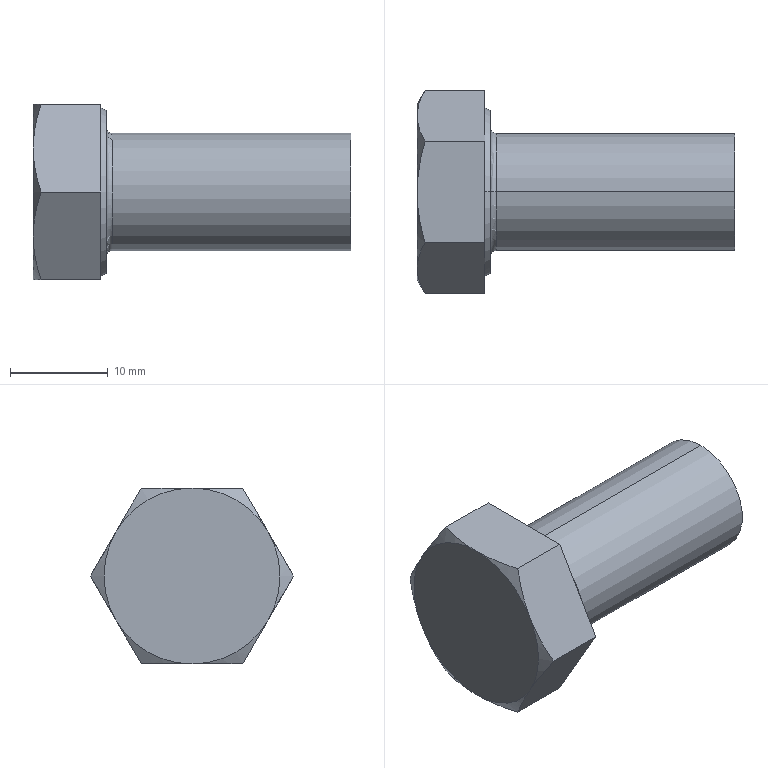Part | SolidWorks | features RevCut 3, Extrusion 1, Fillet 1, LPattern 1, Revolution 1 | 1 solid | 22 faces | box 32.5 x 20.785 x 18 mm | volume 4896 mm3 | plane 10 | cone 8 | torus 2 | cylinder 2 | commonest cylinder face diameters 12 x2
STEP:
#1=CARTESIAN_POINT('',(8.1,0.,6.));
#2=VERTEX_POINT('',#1);
#3=CARTESIAN_POINT('',(8.1,0.,-6.));
#4=VERTEX_POINT('',#3);
#5=CARTESIAN_POINT('',(8.1,0.,0.));
#6=DIRECTION('',(1.,0.,0.));
#7=DIRECTION('',(0.,0.,-1.));
#8=AXIS2_PLACEMENT_3D('',#5,#6,#7);
#9=CIRCLE('',#8,6.);
#10=EDGE_CURVE('',#2,#4,#9,.T.);
#11=ORIENTED_EDGE('',*,*,#10,.F.);
#12=CARTESIAN_POINT('',(7.5,0.,6.6));
#13=VERTEX_POINT('',#12);
#14=CARTESIAN_POINT('',(8.1,0.,6.6));
#15=DIRECTION('',(0.,1.,0.));
#16=DIRECTION('',(0.,0.,1.));
#17=AXIS2_PLACEMENT_3D('',#14,#15,#16);
#18=CIRCLE('',#17,0.6);
#19=EDGE_CURVE('',#2,#13,#18,.T.);
#20=ORIENTED_EDGE('',*,*,#19,.T.);
#21=CARTESIAN_POINT('',(7.5,0.,-6.6));
#22=VERTEX_POINT('',#21);
#23=CARTESIAN_POINT('',(7.5,0.,0.));
#24=DIRECTION('',(-1.,0.,0.));
#25=DIRECTION('',(0.,0.,-1.));
#26=AXIS2_PLACEMENT_3D('',#23,#24,#25);
#27=CIRCLE('',#26,6.6);
#28=EDGE_CURVE('',#22,#13,#27,.T.);
#29=ORIENTED_EDGE('',*,*,#28,.F.);
#30=CARTESIAN_POINT('',(8.1,0.,-6.6));
#31=DIRECTION('',(0.,-1.,0.));
#32=DIRECTION('',(0.,0.,-1.));
#33=AXIS2_PLACEMENT_3D('',#30,#31,#32);
#34=CIRCLE('',#33,0.6);
#35=EDGE_CURVE('',#4,#22,#34,.T.);
#36=ORIENTED_EDGE('',*,*,#35,.F.);
#37=EDGE_LOOP('',(#11,#20,#29,#36));
#38=FACE_OUTER_BOUND('',#37,.T.);
#39=CARTESIAN_POINT('',(8.1,0.,0.));
#40=DIRECTION('',(1.,0.,0.));
#41=DIRECTION('',(0.,0.,-1.));
#42=AXIS2_PLACEMENT_3D('',#39,#40,#41);
#43=TOROIDAL_SURFACE('',#42,6.6,0.6);
#44=ADVANCED_FACE('',(#38),#43,.F.);
#45=CARTESIAN_POINT('',(32.5,0.,6.));
#46=VERTEX_POINT('',#45);
#47=CARTESIAN_POINT('',(32.5,0.,-6.));
#48=VERTEX_POINT('',#47);
#49=CARTESIAN_POINT('',(32.5,0.,0.));
#50=DIRECTION('',(-1.,0.,0.));
#51=DIRECTION('',(0.,0.,1.));
#52=AXIS2_PLACEMENT_3D('',#49,#50,#51);
#53=CIRCLE('',#52,6.);
#54=EDGE_CURVE('',#46,#48,#53,.T.);
#55=ORIENTED_EDGE('',*,*,#54,.T.);
#56=CARTESIAN_POINT('',(0.,0.,-6.));
#57=DIRECTION('',(-1.,0.,0.));
#58=VECTOR('',#57,1000.);
#59=LINE('',#56,#58);
#60=EDGE_CURVE('',#48,#4,#59,.T.);
#61=ORIENTED_EDGE('',*,*,#60,.T.);
#62=CARTESIAN_POINT('',(8.1,0.,0.));
#63=DIRECTION('',(1.,0.,0.));
#64=DIRECTION('',(0.,0.,-1.));
#65=AXIS2_PLACEMENT_3D('',#62,#63,#64);
#66=CIRCLE('',#65,6.);
#67=EDGE_CURVE('',#4,#2,#66,.T.);
#68=ORIENTED_EDGE('',*,*,#67,.T.);
#69=CARTESIAN_POINT('',(0.,0.,6.));
#70=DIRECTION('',(-1.,0.,0.));
#71=VECTOR('',#70,1000.);
#72=LINE('',#69,#71);
#73=EDGE_CURVE('',#46,#2,#72,.T.);
#74=ORIENTED_EDGE('',*,*,#73,.F.);
#75=EDGE_LOOP('',(#55,#61,#68,#74));
#76=FACE_OUTER_BOUND('',#75,.T.);
#77=CARTESIAN_POINT('',(0.,0.,0.));
#78=DIRECTION('',(-1.,0.,0.));
#79=DIRECTION('',(0.,0.,1.));
#80=AXIS2_PLACEMENT_3D('',#77,#78,#79);
#81=CYLINDRICAL_SURFACE('',#80,6.);
#82=ADVANCED_FACE('',(#76),#81,.T.);
#83=CARTESIAN_POINT('',(7.5,0.,8.315));
#84=VERTEX_POINT('',#83);
#85=CARTESIAN_POINT('',(7.5,0.,-8.315));
#86=VERTEX_POINT('',#85);
#87=CARTESIAN_POINT('',(7.5,0.,0.));
#88=DIRECTION('',(-1.,0.,0.));
#89=DIRECTION('',(0.,0.,1.));
#90=AXIS2_PLACEMENT_3D('',#87,#88,#89);
#91=CIRCLE('',#90,8.315);
#92=EDGE_CURVE('',#84,#86,#91,.T.);
#93=ORIENTED_EDGE('',*,*,#92,.T.);
#94=CARTESIAN_POINT('',(6.9,0.,-8.661));
#95=VERTEX_POINT('',#94);
#96=CARTESIAN_POINT('',(6.9,0.,-8.661));
#97=DIRECTION('',(-0.866,0.,-0.5));
#98=VECTOR('',#97,1000.);
#99=LINE('',#96,#98);
#100=EDGE_CURVE('',#86,#95,#99,.T.);
#101=ORIENTED_EDGE('',*,*,#100,.T.);
#102=CARTESIAN_POINT('',(6.9,0.,8.661));
#103=VERTEX_POINT('',#102);
#104=CARTESIAN_POINT('',(6.9,0.,0.));
#105=DIRECTION('',(-1.,0.,0.));
#106=DIRECTION('',(0.,0.,1.));
#107=AXIS2_PLACEMENT_3D('',#104,#105,#106);
#108=CIRCLE('',#107,8.661);
#109=EDGE_CURVE('',#103,#95,#108,.T.);
#110=ORIENTED_EDGE('',*,*,#109,.F.);
#111=CARTESIAN_POINT('',(6.9,0.,8.661));
#112=DIRECTION('',(-0.866,0.,0.5));
#113=VECTOR('',#112,1000.);
#114=LINE('',#111,#113);
#115=EDGE_CURVE('',#84,#103,#114,.T.);
#116=ORIENTED_EDGE('',*,*,#115,.F.);
#117=EDGE_LOOP('',(#93,#101,#110,#116));
#118=FACE_OUTER_BOUND('',#117,.T.);
#119=CARTESIAN_POINT('',(6.9,0.,0.));
#120=DIRECTION('',(-1.,0.,0.));
#121=DIRECTION('',(0.,0.,1.));
#122=AXIS2_PLACEMENT_3D('',#119,#120,#121);
#123=CONICAL_SURFACE('',#122,8.661,0.5236);
#124=ADVANCED_FACE('',(#118),#123,.T.);
#125=CARTESIAN_POINT('',(6.9,5.196,-9.));
#126=VERTEX_POINT('',#125);
#127=CARTESIAN_POINT('',(6.9,10.392,0.));
#128=VERTEX_POINT('',#127);
#129=CARTESIAN_POINT('',(6.9,5.196,-9.));
#130=DIRECTION('',(0.,0.5,0.866));
#131=VECTOR('',#130,1000.);
#132=LINE('',#129,#131);
#133=EDGE_CURVE('',#126,#128,#132,.T.);
#134=ORIENTED_EDGE('',*,*,#133,.F.);
#135=CARTESIAN_POINT('',(0.8038,5.196,-9.));
#136=VERTEX_POINT('',#135);
#137=CARTESIAN_POINT('',(7.5,5.196,-9.));
#138=DIRECTION('',(-1.,0.,0.));
#139=VECTOR('',#138,1000.);
#140=LINE('',#137,#139);
#141=EDGE_CURVE('',#126,#136,#140,.T.);
#142=ORIENTED_EDGE('',*,*,#141,.T.);
#143=CARTESIAN_POINT('',(0.,7.794,-4.5));
#144=VERTEX_POINT('',#143);
#145=CARTESIAN_POINT('',(0.,7.794,-4.5));
#146=CARTESIAN_POINT('',(0.,7.574,-4.882));
#147=CARTESIAN_POINT('',(0.019,7.352,-5.266));
#148=CARTESIAN_POINT('',(0.09253,6.914,-6.024));
#149=CARTESIAN_POINT('',(0.147,6.697,-6.401));
#150=CARTESIAN_POINT('',(0.357,6.048,-7.525));
#151=CARTESIAN_POINT('',(0.5591,5.62,-8.266));
#152=CARTESIAN_POINT('',(0.8038,5.196,-9.));
#153=B_SPLINE_CURVE_WITH_KNOTS('',3,(#145,#146,#147,#148,#149,#150,#151,#152),.UNSPECIFIED.,.F.,.F.,(4,2,2,4),(0.005258,0.006567,0.007877,0.0105),.UNSPECIFIED.);
#154=EDGE_CURVE('',#144,#136,#153,.T.);
#155=ORIENTED_EDGE('',*,*,#154,.F.);
#156=CARTESIAN_POINT('',(0.8038,10.392,0.));
#157=VERTEX_POINT('',#156);
#158=CARTESIAN_POINT('',(0.8038,10.392,0.));
#159=CARTESIAN_POINT('',(0.5585,9.967,-0.7361));
#160=CARTESIAN_POINT('',(0.3563,9.539,-1.478));
#161=CARTESIAN_POINT('',(0.07661,8.674,-2.976));
#162=CARTESIAN_POINT('',(0.,8.237,-3.733));
#163=CARTESIAN_POINT('',(0.,7.794,-4.5));
#164=B_SPLINE_CURVE_WITH_KNOTS('',3,(#158,#159,#160,#161,#162,#163),.UNSPECIFIED.,.F.,.F.,(4,2,4),(0.000000238,0.002629,0.005258),.UNSPECIFIED.);
#165=EDGE_CURVE('',#157,#144,#164,.T.);
#166=ORIENTED_EDGE('',*,*,#165,.F.);
#167=CARTESIAN_POINT('',(7.5,10.392,0.));
#168=DIRECTION('',(-1.,0.,0.));
#169=VECTOR('',#168,1000.);
#170=LINE('',#167,#169);
#171=EDGE_CURVE('',#128,#157,#170,.T.);
#172=ORIENTED_EDGE('',*,*,#171,.F.);
#173=EDGE_LOOP('',(#134,#142,#155,#166,#172));
#174=FACE_OUTER_BOUND('',#173,.T.);
#175=CARTESIAN_POINT('',(7.5,5.196,-9.));
#176=DIRECTION('',(0.,-0.866,0.5));
#177=DIRECTION('',(0.,-0.5,-0.866));
#178=AXIS2_PLACEMENT_3D('',#175,#176,#177);
#179=PLANE('',#178);
#180=ADVANCED_FACE('',(#174),#179,.F.);
#181=CARTESIAN_POINT('',(6.9,5.196,9.));
#182=VERTEX_POINT('',#181);
#183=CARTESIAN_POINT('',(6.9,10.392,0.));
#184=DIRECTION('',(0.,-0.5,0.866));
#185=VECTOR('',#184,1000.);
#186=LINE('',#183,#185);
#187=EDGE_CURVE('',#128,#182,#186,.T.);
#188=ORIENTED_EDGE('',*,*,#187,.F.);
#189=ORIENTED_EDGE('',*,*,#171,.T.);
#190=CARTESIAN_POINT('',(0.,7.794,4.5));
#191=VERTEX_POINT('',#190);
#192=CARTESIAN_POINT('',(0.,7.794,4.5));
#193=CARTESIAN_POINT('',(0.,8.015,4.118));
#194=CARTESIAN_POINT('',(0.019,8.236,3.734));
#195=CARTESIAN_POINT('',(0.09253,8.674,2.976));
#196=CARTESIAN_POINT('',(0.147,8.892,2.599));
#197=CARTESIAN_POINT('',(0.357,9.541,1.475));
#198=CARTESIAN_POINT('',(0.5591,9.968,0.7343));
#199=CARTESIAN_POINT('',(0.8038,10.392,0.));
#200=B_SPLINE_CURVE_WITH_KNOTS('',3,(#192,#193,#194,#195,#196,#197,#198,#199),.UNSPECIFIED.,.F.,.F.,(4,2,2,4),(0.005258,0.006567,0.007877,0.0105),.UNSPECIFIED.);
#201=EDGE_CURVE('',#191,#157,#200,.T.);
#202=ORIENTED_EDGE('',*,*,#201,.F.);
#203=CARTESIAN_POINT('',(0.8038,5.196,9.));
#204=VERTEX_POINT('',#203);
#205=CARTESIAN_POINT('',(0.8038,5.196,9.));
#206=CARTESIAN_POINT('',(0.5585,5.621,8.264));
#207=CARTESIAN_POINT('',(0.3563,6.049,7.522));
#208=CARTESIAN_POINT('',(0.07661,6.914,6.024));
#209=CARTESIAN_POINT('',(0.,7.352,5.267));
#210=CARTESIAN_POINT('',(0.,7.794,4.5));
#211=B_SPLINE_CURVE_WITH_KNOTS('',3,(#205,#206,#207,#208,#209,#210),.UNSPECIFIED.,.F.,.F.,(4,2,4),(0.000000238,0.002629,0.005258),.UNSPECIFIED.);
#212=EDGE_CURVE('',#204,#191,#211,.T.);
#213=ORIENTED_EDGE('',*,*,#212,.F.);
#214=CARTESIAN_POINT('',(7.5,5.196,9.));
#215=DIRECTION('',(-1.,0.,0.));
#216=VECTOR('',#215,1000.);
#217=LINE('',#214,#216);
#218=EDGE_CURVE('',#182,#204,#217,.T.);
#219=ORIENTED_EDGE('',*,*,#218,.F.);
#220=EDGE_LOOP('',(#188,#189,#202,#213,#219));
#221=FACE_OUTER_BOUND('',#220,.T.);
#222=CARTESIAN_POINT('',(7.5,10.392,0.));
#223=DIRECTION('',(0.,-0.866,-0.5));
#224=DIRECTION('',(0.,0.5,-0.866));
#225=AXIS2_PLACEMENT_3D('',#222,#223,#224);
#226=PLANE('',#225);
#227=ADVANCED_FACE('',(#221),#226,.F.);
#228=CARTESIAN_POINT('',(6.9,-5.196,9.));
#229=VERTEX_POINT('',#228);
#230=CARTESIAN_POINT('',(6.9,5.196,9.));
#231=DIRECTION('',(0.,-1.,0.));
#232=VECTOR('',#231,1000.);
#233=LINE('',#230,#232);
#234=EDGE_CURVE('',#182,#229,#233,.T.);
#235=ORIENTED_EDGE('',*,*,#234,.F.);
#236=ORIENTED_EDGE('',*,*,#218,.T.);
#237=CARTESIAN_POINT('',(0.,0.,9.));
#238=VERTEX_POINT('',#237);
#239=CARTESIAN_POINT('',(0.,0.,9.));
#240=CARTESIAN_POINT('',(0.,0.4401,9.));
#241=CARTESIAN_POINT('',(0.01885,0.8832,9.));
#242=CARTESIAN_POINT('',(0.09319,1.767,9.));
#243=CARTESIAN_POINT('',(0.1482,2.204,9.));
#244=CARTESIAN_POINT('',(0.3593,3.505,9.));
#245=CARTESIAN_POINT('',(0.5612,4.356,9.));
#246=CARTESIAN_POINT('',(0.8038,5.196,9.));
#247=B_SPLINE_CURVE_WITH_KNOTS('',3,(#239,#240,#241,#242,#243,#244,#245,#246),.UNSPECIFIED.,.F.,.F.,(4,2,2,4),(0.01498,0.0163,0.01761,0.02025),.UNSPECIFIED.);
#248=EDGE_CURVE('',#238,#204,#247,.T.);
#249=ORIENTED_EDGE('',*,*,#248,.F.);
#250=CARTESIAN_POINT('',(0.8038,-5.196,9.));
#251=VERTEX_POINT('',#250);
#252=CARTESIAN_POINT('',(0.8038,-5.196,9.));
#253=CARTESIAN_POINT('',(0.5595,-4.35,9.));
#254=CARTESIAN_POINT('',(0.3552,-3.485,9.));
#255=CARTESIAN_POINT('',(0.07569,-1.752,9.));
#256=CARTESIAN_POINT('',(0.,-0.8794,9.));
#257=CARTESIAN_POINT('',(0.,0.,9.));
#258=B_SPLINE_CURVE_WITH_KNOTS('',3,(#252,#253,#254,#255,#256,#257),.UNSPECIFIED.,.F.,.F.,(4,2,4),(0.00972,0.01235,0.01498),.UNSPECIFIED.);
#259=EDGE_CURVE('',#251,#238,#258,.T.);
#260=ORIENTED_EDGE('',*,*,#259,.F.);
#261=CARTESIAN_POINT('',(7.5,-5.196,9.));
#262=DIRECTION('',(-1.,0.,0.));
#263=VECTOR('',#262,1000.);
#264=LINE('',#261,#263);
#265=EDGE_CURVE('',#229,#251,#264,.T.);
#266=ORIENTED_EDGE('',*,*,#265,.F.);
#267=EDGE_LOOP('',(#235,#236,#249,#260,#266));
#268=FACE_OUTER_BOUND('',#267,.T.);
#269=CARTESIAN_POINT('',(7.5,5.196,9.));
#270=DIRECTION('',(0.,0.,-1.));
#271=DIRECTION('',(-1.,0.,0.));
#272=AXIS2_PLACEMENT_3D('',#269,#270,#271);
#273=PLANE('',#272);
#274=ADVANCED_FACE('',(#268),#273,.F.);
#275=CARTESIAN_POINT('',(6.9,-10.392,0.));
#276=VERTEX_POINT('',#275);
#277=CARTESIAN_POINT('',(6.9,-10.392,0.));
#278=DIRECTION('',(0.,-0.5,-0.866));
#279=VECTOR('',#278,1000.);
#280=LINE('',#277,#279);
#281=EDGE_CURVE('',#229,#276,#280,.T.);
#282=ORIENTED_EDGE('',*,*,#281,.F.);
#283=ORIENTED_EDGE('',*,*,#265,.T.);
#284=CARTESIAN_POINT('',(0.,-7.794,4.5));
#285=VERTEX_POINT('',#284);
#286=CARTESIAN_POINT('',(0.,-7.794,4.5));
#287=CARTESIAN_POINT('',(0.,-7.574,4.882));
#288=CARTESIAN_POINT('',(0.019,-7.352,5.266));
#289=CARTESIAN_POINT('',(0.09253,-6.914,6.024));
#290=CARTESIAN_POINT('',(0.147,-6.697,6.401));
#291=CARTESIAN_POINT('',(0.357,-6.048,7.525));
#292=CARTESIAN_POINT('',(0.5591,-5.62,8.266));
#293=CARTESIAN_POINT('',(0.8038,-5.196,9.));
#294=B_SPLINE_CURVE_WITH_KNOTS('',3,(#286,#287,#288,#289,#290,#291,#292,#293),.UNSPECIFIED.,.F.,.F.,(4,2,2,4),(0.005258,0.006567,0.007877,0.0105),.UNSPECIFIED.);
#295=EDGE_CURVE('',#285,#251,#294,.T.);
#296=ORIENTED_EDGE('',*,*,#295,.F.);
#297=CARTESIAN_POINT('',(0.8038,-10.392,0.));
#298=VERTEX_POINT('',#297);
#299=CARTESIAN_POINT('',(0.8038,-10.392,0.));
#300=CARTESIAN_POINT('',(0.5585,-9.967,0.7361));
#301=CARTESIAN_POINT('',(0.3563,-9.539,1.478));
#302=CARTESIAN_POINT('',(0.07661,-8.674,2.976));
#303=CARTESIAN_POINT('',(0.,-8.237,3.733));
#304=CARTESIAN_POINT('',(0.,-7.794,4.5));
#305=B_SPLINE_CURVE_WITH_KNOTS('',3,(#299,#300,#301,#302,#303,#304),.UNSPECIFIED.,.F.,.F.,(4,2,4),(0.000000238,0.002629,0.005258),.UNSPECIFIED.);
#306=EDGE_CURVE('',#298,#285,#305,.T.);
#307=ORIENTED_EDGE('',*,*,#306,.F.);
#308=CARTESIAN_POINT('',(7.5,-10.392,0.));
#309=DIRECTION('',(-1.,0.,0.));
#310=VECTOR('',#309,1000.);
#311=LINE('',#308,#310);
#312=EDGE_CURVE('',#276,#298,#311,.T.);
#313=ORIENTED_EDGE('',*,*,#312,.F.);
#314=EDGE_LOOP('',(#282,#283,#296,#307,#313));
#315=FACE_OUTER_BOUND('',#314,.T.);
#316=CARTESIAN_POINT('',(7.5,-10.392,0.));
#317=DIRECTION('',(0.,0.866,-0.5));
#318=DIRECTION('',(0.,0.5,0.866));
#319=AXIS2_PLACEMENT_3D('',#316,#317,#318);
#320=PLANE('',#319);
#321=ADVANCED_FACE('',(#315),#320,.F.);
#322=CARTESIAN_POINT('',(6.9,-5.196,-9.));
#323=VERTEX_POINT('',#322);
#324=CARTESIAN_POINT('',(6.9,-5.196,-9.));
#325=DIRECTION('',(0.,0.5,-0.866));
#326=VECTOR('',#325,1000.);
#327=LINE('',#324,#326);
#328=EDGE_CURVE('',#276,#323,#327,.T.);
#329=ORIENTED_EDGE('',*,*,#328,.F.);
#330=ORIENTED_EDGE('',*,*,#312,.T.);
#331=CARTESIAN_POINT('',(0.,-7.794,-4.5));
#332=VERTEX_POINT('',#331);
#333=CARTESIAN_POINT('',(0.,-7.794,-4.5));
#334=CARTESIAN_POINT('',(0.,-8.015,-4.118));
#335=CARTESIAN_POINT('',(0.019,-8.236,-3.734));
#336=CARTESIAN_POINT('',(0.09253,-8.674,-2.976));
#337=CARTESIAN_POINT('',(0.147,-8.892,-2.599));
#338=CARTESIAN_POINT('',(0.357,-9.541,-1.475));
#339=CARTESIAN_POINT('',(0.5591,-9.968,-0.7343));
#340=CARTESIAN_POINT('',(0.8038,-10.392,0.));
#341=B_SPLINE_CURVE_WITH_KNOTS('',3,(#333,#334,#335,#336,#337,#338,#339,#340),.UNSPECIFIED.,.F.,.F.,(4,2,2,4),(0.005258,0.006567,0.007877,0.0105),.UNSPECIFIED.);
#342=EDGE_CURVE('',#332,#298,#341,.T.);
#343=ORIENTED_EDGE('',*,*,#342,.F.);
#344=CARTESIAN_POINT('',(0.8038,-5.196,-9.));
#345=VERTEX_POINT('',#344);
#346=CARTESIAN_POINT('',(0.8038,-5.196,-9.));
#347=CARTESIAN_POINT('',(0.5585,-5.621,-8.264));
#348=CARTESIAN_POINT('',(0.3563,-6.049,-7.522));
#349=CARTESIAN_POINT('',(0.07661,-6.914,-6.024));
#350=CARTESIAN_POINT('',(0.,-7.352,-5.267));
#351=CARTESIAN_POINT('',(0.,-7.794,-4.5));
#352=B_SPLINE_CURVE_WITH_KNOTS('',3,(#346,#347,#348,#349,#350,#351),.UNSPECIFIED.,.F.,.F.,(4,2,4),(0.000000238,0.002629,0.005258),.UNSPECIFIED.);
#353=EDGE_CURVE('',#345,#332,#352,.T.);
#354=ORIENTED_EDGE('',*,*,#353,.F.);
#355=CARTESIAN_POINT('',(7.5,-5.196,-9.));
#356=DIRECTION('',(-1.,0.,0.));
#357=VECTOR('',#356,1000.);
#358=LINE('',#355,#357);
#359=EDGE_CURVE('',#323,#345,#358,.T.);
#360=ORIENTED_EDGE('',*,*,#359,.F.);
#361=EDGE_LOOP('',(#329,#330,#343,#354,#360));
#362=FACE_OUTER_BOUND('',#361,.T.);
#363=CARTESIAN_POINT('',(7.5,-5.196,-9.));
#364=DIRECTION('',(0.,0.866,0.5));
#365=DIRECTION('',(0.,-0.5,0.866));
#366=AXIS2_PLACEMENT_3D('',#363,#364,#365);
#367=PLANE('',#366);
#368=ADVANCED_FACE('',(#362),#367,.F.);
#369=CARTESIAN_POINT('',(6.9,5.196,-9.));
#370=DIRECTION('',(0.,1.,0.));
#371=VECTOR('',#370,1000.);
#372=LINE('',#369,#371);
#373=EDGE_CURVE('',#323,#126,#372,.T.);
#374=ORIENTED_EDGE('',*,*,#373,.F.);
#375=ORIENTED_EDGE('',*,*,#359,.T.);
#376=CARTESIAN_POINT('',(0.,0.,-9.));
#377=VERTEX_POINT('',#376);
#378=CARTESIAN_POINT('',(0.,0.,-9.));
#379=CARTESIAN_POINT('',(0.,-0.8794,-9.));
#380=CARTESIAN_POINT('',(0.07569,-1.752,-9.));
#381=CARTESIAN_POINT('',(0.3552,-3.485,-9.));
#382=CARTESIAN_POINT('',(0.5595,-4.35,-9.));
#383=CARTESIAN_POINT('',(0.8038,-5.196,-9.));
#384=B_SPLINE_CURVE_WITH_KNOTS('',3,(#378,#379,#380,#381,#382,#383),.UNSPECIFIED.,.F.,.F.,(4,2,4),(0.03045,0.03308,0.03571),.UNSPECIFIED.);
#385=EDGE_CURVE('',#377,#345,#384,.T.);
#386=ORIENTED_EDGE('',*,*,#385,.F.);
#387=CARTESIAN_POINT('',(0.8038,5.196,-9.));
#388=CARTESIAN_POINT('',(0.5612,4.356,-9.));
#389=CARTESIAN_POINT('',(0.3593,3.505,-9.));
#390=CARTESIAN_POINT('',(0.1482,2.204,-9.));
#391=CARTESIAN_POINT('',(0.09319,1.767,-9.));
#392=CARTESIAN_POINT('',(0.01885,0.8832,-9.));
#393=CARTESIAN_POINT('',(0.,0.4401,-9.));
#394=CARTESIAN_POINT('',(0.,0.,-9.));
#395=B_SPLINE_CURVE_WITH_KNOTS('',3,(#387,#388,#389,#390,#391,#392,#393,#394),.UNSPECIFIED.,.F.,.F.,(4,2,2,4),(0.02519,0.02782,0.02914,0.03045),.UNSPECIFIED.);
#396=EDGE_CURVE('',#136,#377,#395,.T.);
#397=ORIENTED_EDGE('',*,*,#396,.F.);
#398=ORIENTED_EDGE('',*,*,#141,.F.);
#399=EDGE_LOOP('',(#374,#375,#386,#397,#398));
#400=FACE_OUTER_BOUND('',#399,.T.);
#401=CARTESIAN_POINT('',(7.5,5.196,-9.));
#402=DIRECTION('',(0.,0.,1.));
#403=DIRECTION('',(0.,-1.,0.));
#404=AXIS2_PLACEMENT_3D('',#401,#402,#403);
#405=PLANE('',#404);
#406=ADVANCED_FACE('',(#400),#405,.F.);
#407=ORIENTED_EDGE('',*,*,#353,.T.);
#408=CARTESIAN_POINT('',(0.,0.,0.));
#409=DIRECTION('',(1.,0.,0.));
#410=DIRECTION('',(0.,0.,-1.));
#411=AXIS2_PLACEMENT_3D('',#408,#409,#410);
#412=CIRCLE('',#411,9.);
#413=EDGE_CURVE('',#332,#377,#412,.T.);
#414=ORIENTED_EDGE('',*,*,#413,.T.);
#415=ORIENTED_EDGE('',*,*,#385,.T.);
#416=EDGE_LOOP('',(#407,#414,#415));
#417=FACE_OUTER_BOUND('',#416,.T.);
#418=CARTESIAN_POINT('',(0.,0.,0.));
#419=DIRECTION('',(1.,0.,0.));
#420=DIRECTION('',(0.,0.,-1.));
#421=AXIS2_PLACEMENT_3D('',#418,#419,#420);
#422=CONICAL_SURFACE('',#421,9.,1.047);
#423=ADVANCED_FACE('',(#417),#422,.T.);
#424=ORIENTED_EDGE('',*,*,#306,.T.);
#425=CARTESIAN_POINT('',(0.,0.,0.));
#426=DIRECTION('',(1.,0.,0.));
#427=DIRECTION('',(0.,0.,-1.));
#428=AXIS2_PLACEMENT_3D('',#425,#426,#427);
#429=CIRCLE('',#428,9.);
#430=EDGE_CURVE('',#285,#332,#429,.T.);
#431=ORIENTED_EDGE('',*,*,#430,.T.);
#432=ORIENTED_EDGE('',*,*,#342,.T.);
#433=EDGE_LOOP('',(#424,#431,#432));
#434=FACE_OUTER_BOUND('',#433,.T.);
#435=CARTESIAN_POINT('',(0.,0.,0.));
#436=DIRECTION('',(1.,0.,0.));
#437=DIRECTION('',(0.,0.,-1.));
#438=AXIS2_PLACEMENT_3D('',#435,#436,#437);
#439=CONICAL_SURFACE('',#438,9.,1.047);
#440=ADVANCED_FACE('',(#434),#439,.T.);
#441=ORIENTED_EDGE('',*,*,#259,.T.);
#442=CARTESIAN_POINT('',(0.,0.,0.));
#443=DIRECTION('',(1.,0.,0.));
#444=DIRECTION('',(0.,0.,-1.));
#445=AXIS2_PLACEMENT_3D('',#442,#443,#444);
#446=CIRCLE('',#445,9.);
#447=EDGE_CURVE('',#238,#285,#446,.T.);
#448=ORIENTED_EDGE('',*,*,#447,.T.);
#449=ORIENTED_EDGE('',*,*,#295,.T.);
#450=EDGE_LOOP('',(#441,#448,#449));
#451=FACE_OUTER_BOUND('',#450,.T.);
#452=CARTESIAN_POINT('',(0.,0.,0.));
#453=DIRECTION('',(1.,0.,0.));
#454=DIRECTION('',(0.,0.,-1.));
#455=AXIS2_PLACEMENT_3D('',#452,#453,#454);
#456=CONICAL_SURFACE('',#455,9.,1.047);
#457=ADVANCED_FACE('',(#451),#456,.T.);
#458=ORIENTED_EDGE('',*,*,#248,.T.);
#459=ORIENTED_EDGE('',*,*,#212,.T.);
#460=CARTESIAN_POINT('',(0.,0.,0.));
#461=DIRECTION('',(-1.,0.,0.));
#462=DIRECTION('',(0.,0.,1.));
#463=AXIS2_PLACEMENT_3D('',#460,#461,#462);
#464=CIRCLE('',#463,9.);
#465=EDGE_CURVE('',#238,#191,#464,.T.);
#466=ORIENTED_EDGE('',*,*,#465,.F.);
#467=EDGE_LOOP('',(#458,#459,#466));
#468=FACE_OUTER_BOUND('',#467,.T.);
#469=CARTESIAN_POINT('',(0.,0.,0.));
#470=DIRECTION('',(1.,0.,0.));
#471=DIRECTION('',(0.,0.,-1.));
#472=AXIS2_PLACEMENT_3D('',#469,#470,#471);
#473=CONICAL_SURFACE('',#472,9.,1.047);
#474=ADVANCED_FACE('',(#468),#473,.T.);
#475=ORIENTED_EDGE('',*,*,#201,.T.);
#476=ORIENTED_EDGE('',*,*,#165,.T.);
#477=CARTESIAN_POINT('',(0.,0.,0.));
#478=DIRECTION('',(1.,0.,0.));
#479=DIRECTION('',(0.,0.,-1.));
#480=AXIS2_PLACEMENT_3D('',#477,#478,#479);
#481=CIRCLE('',#480,9.);
#482=EDGE_CURVE('',#144,#191,#481,.T.);
#483=ORIENTED_EDGE('',*,*,#482,.T.);
#484=EDGE_LOOP('',(#475,#476,#483));
#485=FACE_OUTER_BOUND('',#484,.T.);
#486=CARTESIAN_POINT('',(0.,0.,0.));
#487=DIRECTION('',(1.,0.,0.));
#488=DIRECTION('',(0.,0.,-1.));
#489=AXIS2_PLACEMENT_3D('',#486,#487,#488);
#490=CONICAL_SURFACE('',#489,9.,1.047);
#491=ADVANCED_FACE('',(#485),#490,.T.);
#492=ORIENTED_EDGE('',*,*,#154,.T.);
#493=ORIENTED_EDGE('',*,*,#396,.T.);
#494=CARTESIAN_POINT('',(0.,0.,0.));
#495=DIRECTION('',(1.,0.,0.));
#496=DIRECTION('',(0.,0.,-1.));
#497=AXIS2_PLACEMENT_3D('',#494,#495,#496);
#498=CIRCLE('',#497,9.);
#499=EDGE_CURVE('',#377,#144,#498,.T.);
#500=ORIENTED_EDGE('',*,*,#499,.T.);
#501=EDGE_LOOP('',(#492,#493,#500));
#502=FACE_OUTER_BOUND('',#501,.T.);
#503=CARTESIAN_POINT('',(0.,0.,0.));
#504=DIRECTION('',(1.,0.,0.));
#505=DIRECTION('',(0.,0.,-1.));
#506=AXIS2_PLACEMENT_3D('',#503,#504,#505);
#507=CONICAL_SURFACE('',#506,9.,1.047);
#508=ADVANCED_FACE('',(#502),#507,.T.);
#509=ORIENTED_EDGE('',*,*,#499,.F.);
#510=ORIENTED_EDGE('',*,*,#413,.F.);
#511=ORIENTED_EDGE('',*,*,#430,.F.);
#512=ORIENTED_EDGE('',*,*,#447,.F.);
#513=ORIENTED_EDGE('',*,*,#465,.T.);
#514=ORIENTED_EDGE('',*,*,#482,.F.);
#515=EDGE_LOOP('',(#509,#510,#511,#512,#513,#514));
#516=FACE_OUTER_BOUND('',#515,.T.);
#517=CARTESIAN_POINT('',(0.,10.392,0.));
#518=DIRECTION('',(1.,0.,0.));
#519=DIRECTION('',(0.,0.,-1.));
#520=AXIS2_PLACEMENT_3D('',#517,#518,#519);
#521=PLANE('',#520);
#522=ADVANCED_FACE('',(#516),#521,.F.);
#523=ORIENTED_EDGE('',*,*,#109,.T.);
#524=CARTESIAN_POINT('',(6.9,0.,0.));
#525=DIRECTION('',(-1.,0.,0.));
#526=DIRECTION('',(0.,0.,1.));
#527=AXIS2_PLACEMENT_3D('',#524,#525,#526);
#528=CIRCLE('',#527,8.661);
#529=EDGE_CURVE('',#95,#103,#528,.T.);
#530=ORIENTED_EDGE('',*,*,#529,.T.);
#531=EDGE_LOOP('',(#523,#530));
#532=FACE_BOUND('',#531,.T.);
#533=ORIENTED_EDGE('',*,*,#133,.T.);
#534=ORIENTED_EDGE('',*,*,#187,.T.);
#535=ORIENTED_EDGE('',*,*,#234,.T.);
#536=ORIENTED_EDGE('',*,*,#281,.T.);
#537=ORIENTED_EDGE('',*,*,#328,.T.);
#538=ORIENTED_EDGE('',*,*,#373,.T.);
#539=EDGE_LOOP('',(#533,#534,#535,#536,#537,#538));
#540=FACE_OUTER_BOUND('',#539,.T.);
#541=CARTESIAN_POINT('',(6.9,8.661,0.));
#542=DIRECTION('',(1.,0.,0.));
#543=DIRECTION('',(0.,0.,-1.));
#544=AXIS2_PLACEMENT_3D('',#541,#542,#543);
#545=PLANE('',#544);
#546=ADVANCED_FACE('',(#532,#540),#545,.T.);
#547=ORIENTED_EDGE('',*,*,#100,.F.);
#548=CARTESIAN_POINT('',(7.5,0.,0.));
#549=DIRECTION('',(-1.,0.,0.));
#550=DIRECTION('',(0.,0.,1.));
#551=AXIS2_PLACEMENT_3D('',#548,#549,#550);
#552=CIRCLE('',#551,8.315);
#553=EDGE_CURVE('',#86,#84,#552,.T.);
#554=ORIENTED_EDGE('',*,*,#553,.T.);
#555=ORIENTED_EDGE('',*,*,#115,.T.);
#556=ORIENTED_EDGE('',*,*,#529,.F.);
#557=EDGE_LOOP('',(#547,#554,#555,#556));
#558=FACE_OUTER_BOUND('',#557,.T.);
#559=CARTESIAN_POINT('',(6.9,0.,0.));
#560=DIRECTION('',(-1.,0.,0.));
#561=DIRECTION('',(0.,0.,1.));
#562=AXIS2_PLACEMENT_3D('',#559,#560,#561);
#563=CONICAL_SURFACE('',#562,8.661,0.5236);
#564=ADVANCED_FACE('',(#558),#563,.T.);
#565=ORIENTED_EDGE('',*,*,#54,.F.);
#566=CARTESIAN_POINT('',(32.5,0.,0.));
#567=DIRECTION('',(-1.,0.,0.));
#568=DIRECTION('',(0.,0.,1.));
#569=AXIS2_PLACEMENT_3D('',#566,#567,#568);
#570=CIRCLE('',#569,6.);
#571=EDGE_CURVE('',#48,#46,#570,.T.);
#572=ORIENTED_EDGE('',*,*,#571,.F.);
#573=EDGE_LOOP('',(#565,#572));
#574=FACE_OUTER_BOUND('',#573,.T.);
#575=CARTESIAN_POINT('',(32.5,0.,0.));
#576=DIRECTION('',(-1.,0.,0.));
#577=DIRECTION('',(0.,0.,1.));
#578=AXIS2_PLACEMENT_3D('',#575,#576,#577);
#579=PLANE('',#578);
#580=ADVANCED_FACE('',(#574),#579,.F.);
#581=ORIENTED_EDGE('',*,*,#60,.F.);
#582=ORIENTED_EDGE('',*,*,#571,.T.);
#583=ORIENTED_EDGE('',*,*,#73,.T.);
#584=ORIENTED_EDGE('',*,*,#10,.T.);
#585=EDGE_LOOP('',(#581,#582,#583,#584));
#586=FACE_OUTER_BOUND('',#585,.T.);
#587=CARTESIAN_POINT('',(0.,0.,0.));
#588=DIRECTION('',(-1.,0.,0.));
#589=DIRECTION('',(0.,0.,1.));
#590=AXIS2_PLACEMENT_3D('',#587,#588,#589);
#591=CYLINDRICAL_SURFACE('',#590,6.);
#592=ADVANCED_FACE('',(#586),#591,.T.);
#593=ORIENTED_EDGE('',*,*,#28,.T.);
#594=CARTESIAN_POINT('',(7.5,0.,0.));
#595=DIRECTION('',(-1.,0.,0.));
#596=DIRECTION('',(0.,0.,-1.));
#597=AXIS2_PLACEMENT_3D('',#594,#595,#596);
#598=CIRCLE('',#597,6.6);
#599=EDGE_CURVE('',#13,#22,#598,.T.);
#600=ORIENTED_EDGE('',*,*,#599,.T.);
#601=EDGE_LOOP('',(#593,#600));
#602=FACE_BOUND('',#601,.T.);
#603=ORIENTED_EDGE('',*,*,#92,.F.);
#604=ORIENTED_EDGE('',*,*,#553,.F.);
#605=EDGE_LOOP('',(#603,#604));
#606=FACE_OUTER_BOUND('',#605,.T.);
#607=CARTESIAN_POINT('',(7.5,10.392,0.));
#608=DIRECTION('',(1.,0.,0.));
#609=DIRECTION('',(0.,0.,-1.));
#610=AXIS2_PLACEMENT_3D('',#607,#608,#609);
#611=PLANE('',#610);
#612=ADVANCED_FACE('',(#602,#606),#611,.T.);
#613=ORIENTED_EDGE('',*,*,#19,.F.);
#614=ORIENTED_EDGE('',*,*,#67,.F.);
#615=ORIENTED_EDGE('',*,*,#35,.T.);
#616=ORIENTED_EDGE('',*,*,#599,.F.);
#617=EDGE_LOOP('',(#613,#614,#615,#616));
#618=FACE_OUTER_BOUND('',#617,.T.);
#619=CARTESIAN_POINT('',(8.1,0.,0.));
#620=DIRECTION('',(1.,0.,0.));
#621=DIRECTION('',(0.,0.,-1.));
#622=AXIS2_PLACEMENT_3D('',#619,#620,#621);
#623=TOROIDAL_SURFACE('',#622,6.6,0.6);
#624=ADVANCED_FACE('',(#618),#623,.F.);
#625=CLOSED_SHELL('',(#44,#82,#124,#180,#227,#274,#321,#368,#406,#423,#440,#457,#474,#491,#508,#522,#546,#564,#580,#592,#612,#624));
#626=MANIFOLD_SOLID_BREP('',#625);
#627=CARTESIAN_POINT('',(0.,0.,0.));
#628=DIRECTION('',(0.,0.,1.));
#629=DIRECTION('',(1.,0.,0.));
#630=AXIS2_PLACEMENT_3D('',#627,#628,#629);
#631=(LENGTH_UNIT()NAMED_UNIT(*)SI_UNIT(.MILLI.,.METRE.));
#632=UNCERTAINTY_MEASURE_WITH_UNIT(LENGTH_MEASURE(0.00001),#631,'','');
#633=(NAMED_UNIT(*)PLANE_ANGLE_UNIT()SI_UNIT($,.RADIAN.));
#634=(NAMED_UNIT(*)SI_UNIT($,.STERADIAN.)SOLID_ANGLE_UNIT());
#635=(GEOMETRIC_REPRESENTATION_CONTEXT(3)GLOBAL_UNCERTAINTY_ASSIGNED_CONTEXT((#632))GLOBAL_UNIT_ASSIGNED_CONTEXT((#631,#633,#634))REPRESENTATION_CONTEXT('',''));
#636=ADVANCED_BREP_SHAPE_REPRESENTATION('',(#626,#630),#635);